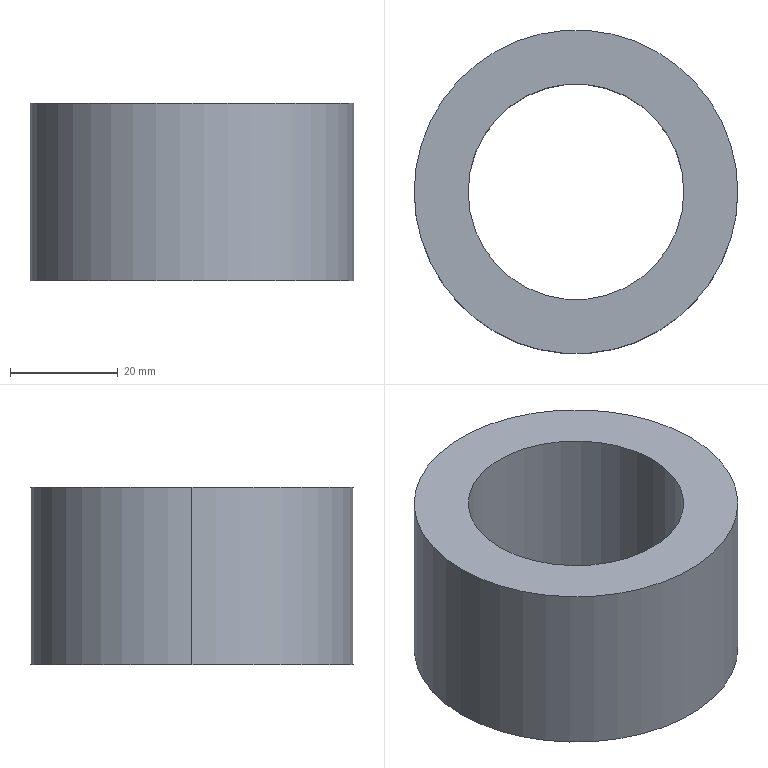Part | STEP file | Shaft retaining ring | 1 solid | 6 faces | box 60 x 60 x 33 mm | volume 51836 mm3 | cylinder 4 | plane 2 | commonest cylinder face diameters 40 x2 60 x2
STEP:
#1=CARTESIAN_POINT('',(0.,0.,0.));
#2=DIRECTION('',(0.,0.,1.));
#3=DIRECTION('',(1.,0.,0.));
#4=AXIS2_PLACEMENT_3D('',#1,#2,#3);
#5=CARTESIAN_POINT('',(-20.,0.,16.5));
#6=VERTEX_POINT('',#5);
#7=CARTESIAN_POINT('',(-20.,0.,-16.5));
#8=VERTEX_POINT('',#7);
#9=CARTESIAN_POINT('',(-20.,0.,16.5));
#10=DIRECTION('',(0.,0.,-1.));
#11=VECTOR('',#10,1.);
#12=LINE('',#9,#11);
#13=CARTESIAN_POINT('',(0.,0.,16.5));
#14=DIRECTION('',(0.,0.,-1.));
#15=DIRECTION('',(-1.,0.,0.));
#16=AXIS2_PLACEMENT_3D('',#13,#14,#15);
#17=CYLINDRICAL_SURFACE('',#16,20.);
#18=CARTESIAN_POINT('',(6.283,0.));
#19=DIRECTION('',(0.,1.));
#20=VECTOR('',#19,1.);
#21=LINE('',#18,#20);
#22=(GEOMETRIC_REPRESENTATION_CONTEXT(2)PARAMETRIC_REPRESENTATION_CONTEXT()REPRESENTATION_CONTEXT('',''));
#23=DEFINITIONAL_REPRESENTATION('',(#21),#22);
#24=PCURVE('',#17,#23);
#25=CARTESIAN_POINT('',(0.,0.,16.5));
#26=DIRECTION('',(0.,0.,-1.));
#27=DIRECTION('',(-1.,0.,0.));
#28=AXIS2_PLACEMENT_3D('',#25,#26,#27);
#29=CYLINDRICAL_SURFACE('',#28,20.);
#30=CARTESIAN_POINT('',(0.,0.));
#31=DIRECTION('',(0.,1.));
#32=VECTOR('',#31,1.);
#33=LINE('',#30,#32);
#34=(GEOMETRIC_REPRESENTATION_CONTEXT(2)PARAMETRIC_REPRESENTATION_CONTEXT()REPRESENTATION_CONTEXT('',''));
#35=DEFINITIONAL_REPRESENTATION('',(#33),#34);
#36=PCURVE('',#29,#35);
#37=SURFACE_CURVE('',#12,(#24,#36),.PCURVE_S1.);
#38=EDGE_CURVE('',#6,#8,#37,.T.);
#39=ORIENTED_EDGE('',*,*,#38,.T.);
#40=CARTESIAN_POINT('',(20.,0.,-16.5));
#41=VERTEX_POINT('',#40);
#42=CARTESIAN_POINT('',(0.,0.,-16.5));
#43=DIRECTION('',(0.,0.,1.));
#44=DIRECTION('',(1.,0.,0.));
#45=AXIS2_PLACEMENT_3D('',#42,#43,#44);
#46=CIRCLE('',#45,20.);
#47=CARTESIAN_POINT('',(9.425,33.));
#48=DIRECTION('',(-1.,0.));
#49=VECTOR('',#48,1.);
#50=LINE('',#47,#49);
#51=(GEOMETRIC_REPRESENTATION_CONTEXT(2)PARAMETRIC_REPRESENTATION_CONTEXT()REPRESENTATION_CONTEXT('',''));
#52=DEFINITIONAL_REPRESENTATION('',(#50),#51);
#53=PCURVE('',#17,#52);
#54=CARTESIAN_POINT('',(0.,0.,-16.5));
#55=DIRECTION('',(0.,0.,1.));
#56=DIRECTION('',(1.,0.,0.));
#57=AXIS2_PLACEMENT_3D('',#54,#55,#56);
#58=PLANE('',#57);
#59=CARTESIAN_POINT('',(0.,0.));
#60=DIRECTION('',(1.,0.));
#61=AXIS2_PLACEMENT_2D('',#59,#60);
#62=CIRCLE('',#61,20.);
#63=(GEOMETRIC_REPRESENTATION_CONTEXT(2)PARAMETRIC_REPRESENTATION_CONTEXT()REPRESENTATION_CONTEXT('',''));
#64=DEFINITIONAL_REPRESENTATION('',(#62),#63);
#65=PCURVE('',#58,#64);
#66=SURFACE_CURVE('',#46,(#53,#65),.PCURVE_S1.);
#67=EDGE_CURVE('',#8,#41,#66,.T.);
#68=ORIENTED_EDGE('',*,*,#67,.T.);
#69=CARTESIAN_POINT('',(20.,0.,16.5));
#70=VERTEX_POINT('',#69);
#71=CARTESIAN_POINT('',(20.,0.,16.5));
#72=DIRECTION('',(0.,0.,-1.));
#73=VECTOR('',#72,1.);
#74=LINE('',#71,#73);
#75=CARTESIAN_POINT('',(3.142,0.));
#76=DIRECTION('',(0.,1.));
#77=VECTOR('',#76,1.);
#78=LINE('',#75,#77);
#79=(GEOMETRIC_REPRESENTATION_CONTEXT(2)PARAMETRIC_REPRESENTATION_CONTEXT()REPRESENTATION_CONTEXT('',''));
#80=DEFINITIONAL_REPRESENTATION('',(#78),#79);
#81=PCURVE('',#17,#80);
#82=CARTESIAN_POINT('',(3.142,0.));
#83=DIRECTION('',(0.,1.));
#84=VECTOR('',#83,1.);
#85=LINE('',#82,#84);
#86=(GEOMETRIC_REPRESENTATION_CONTEXT(2)PARAMETRIC_REPRESENTATION_CONTEXT()REPRESENTATION_CONTEXT('',''));
#87=DEFINITIONAL_REPRESENTATION('',(#85),#86);
#88=PCURVE('',#29,#87);
#89=SURFACE_CURVE('',#74,(#81,#88),.PCURVE_S1.);
#90=EDGE_CURVE('',#70,#41,#89,.T.);
#91=ORIENTED_EDGE('',*,*,#90,.F.);
#92=CARTESIAN_POINT('',(0.,0.,16.5));
#93=DIRECTION('',(0.,0.,1.));
#94=DIRECTION('',(1.,0.,0.));
#95=AXIS2_PLACEMENT_3D('',#92,#93,#94);
#96=CIRCLE('',#95,20.);
#97=CARTESIAN_POINT('',(9.425,0.));
#98=DIRECTION('',(-1.,0.));
#99=VECTOR('',#98,1.);
#100=LINE('',#97,#99);
#101=(GEOMETRIC_REPRESENTATION_CONTEXT(2)PARAMETRIC_REPRESENTATION_CONTEXT()REPRESENTATION_CONTEXT('',''));
#102=DEFINITIONAL_REPRESENTATION('',(#100),#101);
#103=PCURVE('',#17,#102);
#104=CARTESIAN_POINT('',(0.,0.,16.5));
#105=DIRECTION('',(0.,0.,1.));
#106=DIRECTION('',(1.,0.,0.));
#107=AXIS2_PLACEMENT_3D('',#104,#105,#106);
#108=PLANE('',#107);
#109=CARTESIAN_POINT('',(0.,0.));
#110=DIRECTION('',(1.,0.));
#111=AXIS2_PLACEMENT_2D('',#109,#110);
#112=CIRCLE('',#111,20.);
#113=(GEOMETRIC_REPRESENTATION_CONTEXT(2)PARAMETRIC_REPRESENTATION_CONTEXT()REPRESENTATION_CONTEXT('',''));
#114=DEFINITIONAL_REPRESENTATION('',(#112),#113);
#115=PCURVE('',#108,#114);
#116=SURFACE_CURVE('',#96,(#103,#115),.PCURVE_S1.);
#117=EDGE_CURVE('',#6,#70,#116,.T.);
#118=ORIENTED_EDGE('',*,*,#117,.F.);
#119=EDGE_LOOP('',(#39,#68,#91,#118));
#120=FACE_BOUND('',#119,.F.);
#121=ADVANCED_FACE('',(#120),#17,.F.);
#122=CARTESIAN_POINT('',(30.,0.,16.5));
#123=VERTEX_POINT('',#122);
#124=CARTESIAN_POINT('',(-30.,0.,16.5));
#125=VERTEX_POINT('',#124);
#126=CARTESIAN_POINT('',(0.,0.,16.5));
#127=DIRECTION('',(0.,0.,1.));
#128=DIRECTION('',(1.,0.,0.));
#129=AXIS2_PLACEMENT_3D('',#126,#127,#128);
#130=CIRCLE('',#129,30.);
#131=CARTESIAN_POINT('',(0.,0.,16.5));
#132=DIRECTION('',(0.,0.,-1.));
#133=DIRECTION('',(-1.,0.,0.));
#134=AXIS2_PLACEMENT_3D('',#131,#132,#133);
#135=CYLINDRICAL_SURFACE('',#134,30.);
#136=CARTESIAN_POINT('',(3.142,0.));
#137=DIRECTION('',(-1.,0.));
#138=VECTOR('',#137,1.);
#139=LINE('',#136,#138);
#140=(GEOMETRIC_REPRESENTATION_CONTEXT(2)PARAMETRIC_REPRESENTATION_CONTEXT()REPRESENTATION_CONTEXT('',''));
#141=DEFINITIONAL_REPRESENTATION('',(#139),#140);
#142=PCURVE('',#135,#141);
#143=CARTESIAN_POINT('',(0.,0.));
#144=DIRECTION('',(1.,0.));
#145=AXIS2_PLACEMENT_2D('',#143,#144);
#146=CIRCLE('',#145,30.);
#147=(GEOMETRIC_REPRESENTATION_CONTEXT(2)PARAMETRIC_REPRESENTATION_CONTEXT()REPRESENTATION_CONTEXT('',''));
#148=DEFINITIONAL_REPRESENTATION('',(#146),#147);
#149=PCURVE('',#108,#148);
#150=SURFACE_CURVE('',#130,(#142,#149),.PCURVE_S1.);
#151=EDGE_CURVE('',#123,#125,#150,.T.);
#152=ORIENTED_EDGE('',*,*,#151,.F.);
#153=CARTESIAN_POINT('',(30.,0.,-16.5));
#154=VERTEX_POINT('',#153);
#155=CARTESIAN_POINT('',(30.,0.,16.5));
#156=DIRECTION('',(0.,0.,-1.));
#157=VECTOR('',#156,1.);
#158=LINE('',#155,#157);
#159=CARTESIAN_POINT('',(3.142,0.));
#160=DIRECTION('',(0.,1.));
#161=VECTOR('',#160,1.);
#162=LINE('',#159,#161);
#163=(GEOMETRIC_REPRESENTATION_CONTEXT(2)PARAMETRIC_REPRESENTATION_CONTEXT()REPRESENTATION_CONTEXT('',''));
#164=DEFINITIONAL_REPRESENTATION('',(#162),#163);
#165=PCURVE('',#135,#164);
#166=CARTESIAN_POINT('',(0.,0.,16.5));
#167=DIRECTION('',(0.,0.,-1.));
#168=DIRECTION('',(-1.,0.,0.));
#169=AXIS2_PLACEMENT_3D('',#166,#167,#168);
#170=CYLINDRICAL_SURFACE('',#169,30.);
#171=CARTESIAN_POINT('',(3.142,0.));
#172=DIRECTION('',(0.,1.));
#173=VECTOR('',#172,1.);
#174=LINE('',#171,#173);
#175=(GEOMETRIC_REPRESENTATION_CONTEXT(2)PARAMETRIC_REPRESENTATION_CONTEXT()REPRESENTATION_CONTEXT('',''));
#176=DEFINITIONAL_REPRESENTATION('',(#174),#175);
#177=PCURVE('',#170,#176);
#178=SURFACE_CURVE('',#158,(#165,#177),.PCURVE_S1.);
#179=EDGE_CURVE('',#123,#154,#178,.T.);
#180=ORIENTED_EDGE('',*,*,#179,.T.);
#181=CARTESIAN_POINT('',(-30.,0.,-16.5));
#182=VERTEX_POINT('',#181);
#183=CARTESIAN_POINT('',(0.,0.,-16.5));
#184=DIRECTION('',(0.,0.,1.));
#185=DIRECTION('',(1.,0.,0.));
#186=AXIS2_PLACEMENT_3D('',#183,#184,#185);
#187=CIRCLE('',#186,30.);
#188=CARTESIAN_POINT('',(3.142,33.));
#189=DIRECTION('',(-1.,0.));
#190=VECTOR('',#189,1.);
#191=LINE('',#188,#190);
#192=(GEOMETRIC_REPRESENTATION_CONTEXT(2)PARAMETRIC_REPRESENTATION_CONTEXT()REPRESENTATION_CONTEXT('',''));
#193=DEFINITIONAL_REPRESENTATION('',(#191),#192);
#194=PCURVE('',#135,#193);
#195=CARTESIAN_POINT('',(0.,0.));
#196=DIRECTION('',(1.,0.));
#197=AXIS2_PLACEMENT_2D('',#195,#196);
#198=CIRCLE('',#197,30.);
#199=(GEOMETRIC_REPRESENTATION_CONTEXT(2)PARAMETRIC_REPRESENTATION_CONTEXT()REPRESENTATION_CONTEXT('',''));
#200=DEFINITIONAL_REPRESENTATION('',(#198),#199);
#201=PCURVE('',#58,#200);
#202=SURFACE_CURVE('',#187,(#194,#201),.PCURVE_S1.);
#203=EDGE_CURVE('',#154,#182,#202,.T.);
#204=ORIENTED_EDGE('',*,*,#203,.T.);
#205=CARTESIAN_POINT('',(-30.,0.,16.5));
#206=DIRECTION('',(0.,0.,-1.));
#207=VECTOR('',#206,1.);
#208=LINE('',#205,#207);
#209=CARTESIAN_POINT('',(0.,0.));
#210=DIRECTION('',(0.,1.));
#211=VECTOR('',#210,1.);
#212=LINE('',#209,#211);
#213=(GEOMETRIC_REPRESENTATION_CONTEXT(2)PARAMETRIC_REPRESENTATION_CONTEXT()REPRESENTATION_CONTEXT('',''));
#214=DEFINITIONAL_REPRESENTATION('',(#212),#213);
#215=PCURVE('',#135,#214);
#216=CARTESIAN_POINT('',(6.283,0.));
#217=DIRECTION('',(0.,1.));
#218=VECTOR('',#217,1.);
#219=LINE('',#216,#218);
#220=(GEOMETRIC_REPRESENTATION_CONTEXT(2)PARAMETRIC_REPRESENTATION_CONTEXT()REPRESENTATION_CONTEXT('',''));
#221=DEFINITIONAL_REPRESENTATION('',(#219),#220);
#222=PCURVE('',#170,#221);
#223=SURFACE_CURVE('',#208,(#215,#222),.PCURVE_S1.);
#224=EDGE_CURVE('',#125,#182,#223,.T.);
#225=ORIENTED_EDGE('',*,*,#224,.F.);
#226=EDGE_LOOP('',(#152,#180,#204,#225));
#227=FACE_BOUND('',#226,.T.);
#228=ADVANCED_FACE('',(#227),#135,.T.);
#229=CARTESIAN_POINT('',(0.,0.,16.5));
#230=DIRECTION('',(0.,0.,1.));
#231=DIRECTION('',(1.,0.,0.));
#232=AXIS2_PLACEMENT_3D('',#229,#230,#231);
#233=CIRCLE('',#232,30.);
#234=CARTESIAN_POINT('',(0.,0.));
#235=DIRECTION('',(1.,0.));
#236=AXIS2_PLACEMENT_2D('',#234,#235);
#237=CIRCLE('',#236,30.);
#238=(GEOMETRIC_REPRESENTATION_CONTEXT(2)PARAMETRIC_REPRESENTATION_CONTEXT()REPRESENTATION_CONTEXT('',''));
#239=DEFINITIONAL_REPRESENTATION('',(#237),#238);
#240=PCURVE('',#108,#239);
#241=CARTESIAN_POINT('',(9.425,0.));
#242=DIRECTION('',(-1.,0.));
#243=VECTOR('',#242,1.);
#244=LINE('',#241,#243);
#245=(GEOMETRIC_REPRESENTATION_CONTEXT(2)PARAMETRIC_REPRESENTATION_CONTEXT()REPRESENTATION_CONTEXT('',''));
#246=DEFINITIONAL_REPRESENTATION('',(#244),#245);
#247=PCURVE('',#170,#246);
#248=SURFACE_CURVE('',#233,(#240,#247),.PCURVE_S1.);
#249=EDGE_CURVE('',#125,#123,#248,.T.);
#250=ORIENTED_EDGE('',*,*,#249,.T.);
#251=ORIENTED_EDGE('',*,*,#151,.T.);
#252=EDGE_LOOP('',(#250,#251));
#253=FACE_BOUND('',#252,.T.);
#254=ORIENTED_EDGE('',*,*,#117,.F.);
#255=CARTESIAN_POINT('',(0.,0.,16.5));
#256=DIRECTION('',(0.,0.,1.));
#257=DIRECTION('',(1.,0.,0.));
#258=AXIS2_PLACEMENT_3D('',#255,#256,#257);
#259=CIRCLE('',#258,20.);
#260=CARTESIAN_POINT('',(0.,0.));
#261=DIRECTION('',(1.,0.));
#262=AXIS2_PLACEMENT_2D('',#260,#261);
#263=CIRCLE('',#262,20.);
#264=(GEOMETRIC_REPRESENTATION_CONTEXT(2)PARAMETRIC_REPRESENTATION_CONTEXT()REPRESENTATION_CONTEXT('',''));
#265=DEFINITIONAL_REPRESENTATION('',(#263),#264);
#266=PCURVE('',#108,#265);
#267=CARTESIAN_POINT('',(3.142,0.));
#268=DIRECTION('',(-1.,0.));
#269=VECTOR('',#268,1.);
#270=LINE('',#267,#269);
#271=(GEOMETRIC_REPRESENTATION_CONTEXT(2)PARAMETRIC_REPRESENTATION_CONTEXT()REPRESENTATION_CONTEXT('',''));
#272=DEFINITIONAL_REPRESENTATION('',(#270),#271);
#273=PCURVE('',#29,#272);
#274=SURFACE_CURVE('',#259,(#266,#273),.PCURVE_S1.);
#275=EDGE_CURVE('',#70,#6,#274,.T.);
#276=ORIENTED_EDGE('',*,*,#275,.F.);
#277=EDGE_LOOP('',(#254,#276));
#278=FACE_BOUND('',#277,.T.);
#279=ADVANCED_FACE('',(#253,#278),#108,.T.);
#280=CARTESIAN_POINT('',(0.,0.,-16.5));
#281=DIRECTION('',(0.,0.,1.));
#282=DIRECTION('',(1.,0.,0.));
#283=AXIS2_PLACEMENT_3D('',#280,#281,#282);
#284=CIRCLE('',#283,30.);
#285=CARTESIAN_POINT('',(0.,0.));
#286=DIRECTION('',(1.,0.));
#287=AXIS2_PLACEMENT_2D('',#285,#286);
#288=CIRCLE('',#287,30.);
#289=(GEOMETRIC_REPRESENTATION_CONTEXT(2)PARAMETRIC_REPRESENTATION_CONTEXT()REPRESENTATION_CONTEXT('',''));
#290=DEFINITIONAL_REPRESENTATION('',(#288),#289);
#291=PCURVE('',#58,#290);
#292=CARTESIAN_POINT('',(9.425,33.));
#293=DIRECTION('',(-1.,0.));
#294=VECTOR('',#293,1.);
#295=LINE('',#292,#294);
#296=(GEOMETRIC_REPRESENTATION_CONTEXT(2)PARAMETRIC_REPRESENTATION_CONTEXT()REPRESENTATION_CONTEXT('',''));
#297=DEFINITIONAL_REPRESENTATION('',(#295),#296);
#298=PCURVE('',#170,#297);
#299=SURFACE_CURVE('',#284,(#291,#298),.PCURVE_S1.);
#300=EDGE_CURVE('',#182,#154,#299,.T.);
#301=ORIENTED_EDGE('',*,*,#300,.F.);
#302=ORIENTED_EDGE('',*,*,#203,.F.);
#303=EDGE_LOOP('',(#301,#302));
#304=FACE_BOUND('',#303,.T.);
#305=ORIENTED_EDGE('',*,*,#67,.T.);
#306=CARTESIAN_POINT('',(0.,0.,-16.5));
#307=DIRECTION('',(0.,0.,1.));
#308=DIRECTION('',(1.,0.,0.));
#309=AXIS2_PLACEMENT_3D('',#306,#307,#308);
#310=CIRCLE('',#309,20.);
#311=CARTESIAN_POINT('',(0.,0.));
#312=DIRECTION('',(1.,0.));
#313=AXIS2_PLACEMENT_2D('',#311,#312);
#314=CIRCLE('',#313,20.);
#315=(GEOMETRIC_REPRESENTATION_CONTEXT(2)PARAMETRIC_REPRESENTATION_CONTEXT()REPRESENTATION_CONTEXT('',''));
#316=DEFINITIONAL_REPRESENTATION('',(#314),#315);
#317=PCURVE('',#58,#316);
#318=CARTESIAN_POINT('',(3.142,33.));
#319=DIRECTION('',(-1.,0.));
#320=VECTOR('',#319,1.);
#321=LINE('',#318,#320);
#322=(GEOMETRIC_REPRESENTATION_CONTEXT(2)PARAMETRIC_REPRESENTATION_CONTEXT()REPRESENTATION_CONTEXT('',''));
#323=DEFINITIONAL_REPRESENTATION('',(#321),#322);
#324=PCURVE('',#29,#323);
#325=SURFACE_CURVE('',#310,(#317,#324),.PCURVE_S1.);
#326=EDGE_CURVE('',#41,#8,#325,.T.);
#327=ORIENTED_EDGE('',*,*,#326,.T.);
#328=EDGE_LOOP('',(#305,#327));
#329=FACE_BOUND('',#328,.T.);
#330=ADVANCED_FACE('',(#304,#329),#58,.F.);
#331=ORIENTED_EDGE('',*,*,#179,.F.);
#332=ORIENTED_EDGE('',*,*,#249,.F.);
#333=ORIENTED_EDGE('',*,*,#224,.T.);
#334=ORIENTED_EDGE('',*,*,#300,.T.);
#335=EDGE_LOOP('',(#331,#332,#333,#334));
#336=FACE_BOUND('',#335,.T.);
#337=ADVANCED_FACE('',(#336),#170,.T.);
#338=ORIENTED_EDGE('',*,*,#326,.T.);
#339=ORIENTED_EDGE('',*,*,#38,.F.);
#340=ORIENTED_EDGE('',*,*,#275,.F.);
#341=ORIENTED_EDGE('',*,*,#90,.T.);
#342=EDGE_LOOP('',(#338,#339,#340,#341));
#343=FACE_BOUND('',#342,.F.);
#344=ADVANCED_FACE('',(#343),#29,.F.);
#345=CLOSED_SHELL('',(#121,#228,#279,#330,#337,#344));
#346=MANIFOLD_SOLID_BREP('',#345);
#347=(LENGTH_UNIT()NAMED_UNIT(*)SI_UNIT(.MILLI.,.METRE.));
#348=UNCERTAINTY_MEASURE_WITH_UNIT(LENGTH_MEASURE(0.0000001),#347,'','');
#349=(NAMED_UNIT(*)PLANE_ANGLE_UNIT()SI_UNIT($,.RADIAN.));
#350=(NAMED_UNIT(*)SI_UNIT($,.STERADIAN.)SOLID_ANGLE_UNIT());
#351=(GEOMETRIC_REPRESENTATION_CONTEXT(3)GLOBAL_UNCERTAINTY_ASSIGNED_CONTEXT((#348))GLOBAL_UNIT_ASSIGNED_CONTEXT((#347,#349,#350))REPRESENTATION_CONTEXT('',''));
#352=ADVANCED_BREP_SHAPE_REPRESENTATION('',(#4,#346),#351);